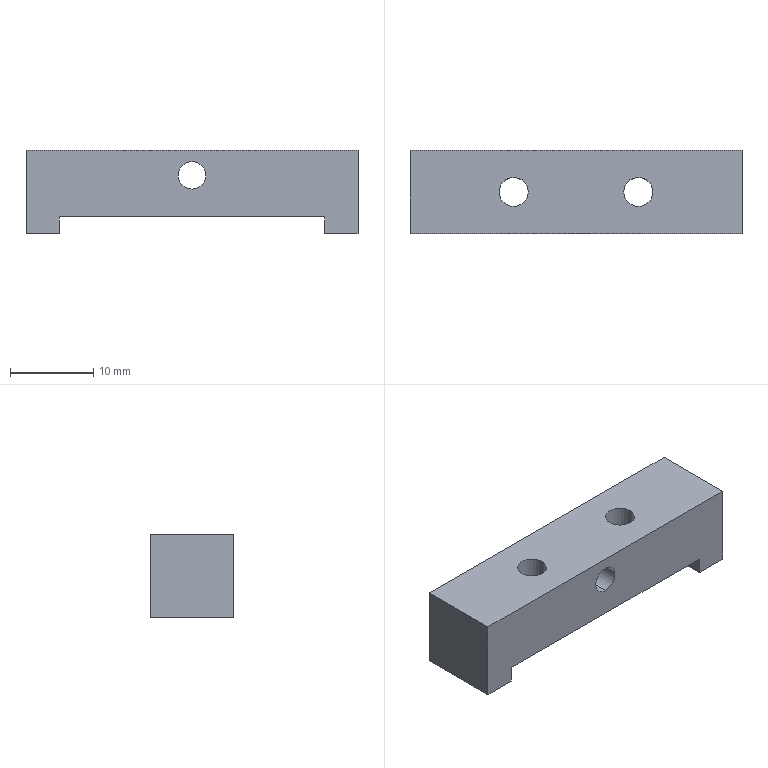Part | STEP file | 11-FG-E04311 | 1 solid | 16 faces | box 40 x 10 x 10 mm | volume 3121 mm3 | plane 10 | cylinder 6 | commonest cylinder face diameters 3.5 x4 3.3 x2
STEP:
#1=CARTESIAN_POINT('',(0.,-5.,5.35));
#2=VERTEX_POINT('',#1);
#3=CARTESIAN_POINT('',(0.,-5.,8.65));
#4=VERTEX_POINT('',#3);
#5=CARTESIAN_POINT('',(0.,-5.,7.));
#6=DIRECTION('',(0.,1.,0.));
#7=DIRECTION('',(0.,0.,1.));
#8=AXIS2_PLACEMENT_3D('',#5,#6,#7);
#9=CIRCLE('',#8,1.65);
#10=EDGE_CURVE('',#2,#4,#9,.T.);
#11=ORIENTED_EDGE('',*,*,#10,.F.);
#12=CARTESIAN_POINT('',(0.,5.,5.35));
#13=VERTEX_POINT('',#12);
#14=CARTESIAN_POINT('',(0.,5.,5.35));
#15=DIRECTION('',(0.,1.,0.));
#16=VECTOR('',#15,1000.);
#17=LINE('',#14,#16);
#18=EDGE_CURVE('',#2,#13,#17,.T.);
#19=ORIENTED_EDGE('',*,*,#18,.T.);
#20=CARTESIAN_POINT('',(0.,5.,8.65));
#21=VERTEX_POINT('',#20);
#22=CARTESIAN_POINT('',(0.,5.,7.));
#23=DIRECTION('',(0.,1.,0.));
#24=DIRECTION('',(0.,0.,1.));
#25=AXIS2_PLACEMENT_3D('',#22,#23,#24);
#26=CIRCLE('',#25,1.65);
#27=EDGE_CURVE('',#13,#21,#26,.T.);
#28=ORIENTED_EDGE('',*,*,#27,.T.);
#29=CARTESIAN_POINT('',(0.,5.,8.65));
#30=DIRECTION('',(0.,1.,0.));
#31=VECTOR('',#30,1000.);
#32=LINE('',#29,#31);
#33=EDGE_CURVE('',#4,#21,#32,.T.);
#34=ORIENTED_EDGE('',*,*,#33,.F.);
#35=EDGE_LOOP('',(#11,#19,#28,#34));
#36=FACE_OUTER_BOUND('',#35,.T.);
#37=CARTESIAN_POINT('',(0.,5.,7.));
#38=DIRECTION('',(0.,1.,0.));
#39=DIRECTION('',(0.,0.,1.));
#40=AXIS2_PLACEMENT_3D('',#37,#38,#39);
#41=CYLINDRICAL_SURFACE('',#40,1.65);
#42=ADVANCED_FACE('',(#36),#41,.F.);
#43=CARTESIAN_POINT('',(5.75,0.,2.));
#44=VERTEX_POINT('',#43);
#45=CARTESIAN_POINT('',(9.25,0.,2.));
#46=VERTEX_POINT('',#45);
#47=CARTESIAN_POINT('',(7.5,0.,2.));
#48=DIRECTION('',(0.,0.,1.));
#49=DIRECTION('',(1.,0.,0.));
#50=AXIS2_PLACEMENT_3D('',#47,#48,#49);
#51=CIRCLE('',#50,1.75);
#52=EDGE_CURVE('',#44,#46,#51,.T.);
#53=ORIENTED_EDGE('',*,*,#52,.F.);
#54=CARTESIAN_POINT('',(5.75,0.,10.));
#55=VERTEX_POINT('',#54);
#56=CARTESIAN_POINT('',(5.75,0.,2.));
#57=DIRECTION('',(0.,0.,1.));
#58=VECTOR('',#57,1000.);
#59=LINE('',#56,#58);
#60=EDGE_CURVE('',#44,#55,#59,.T.);
#61=ORIENTED_EDGE('',*,*,#60,.T.);
#62=CARTESIAN_POINT('',(9.25,0.,10.));
#63=VERTEX_POINT('',#62);
#64=CARTESIAN_POINT('',(7.5,0.,10.));
#65=DIRECTION('',(0.,0.,1.));
#66=DIRECTION('',(1.,0.,0.));
#67=AXIS2_PLACEMENT_3D('',#64,#65,#66);
#68=CIRCLE('',#67,1.75);
#69=EDGE_CURVE('',#55,#63,#68,.T.);
#70=ORIENTED_EDGE('',*,*,#69,.T.);
#71=CARTESIAN_POINT('',(9.25,0.,2.));
#72=DIRECTION('',(0.,0.,1.));
#73=VECTOR('',#72,1000.);
#74=LINE('',#71,#73);
#75=EDGE_CURVE('',#46,#63,#74,.T.);
#76=ORIENTED_EDGE('',*,*,#75,.F.);
#77=EDGE_LOOP('',(#53,#61,#70,#76));
#78=FACE_OUTER_BOUND('',#77,.T.);
#79=CARTESIAN_POINT('',(7.5,0.,2.));
#80=DIRECTION('',(0.,0.,1.));
#81=DIRECTION('',(1.,0.,0.));
#82=AXIS2_PLACEMENT_3D('',#79,#80,#81);
#83=CYLINDRICAL_SURFACE('',#82,1.75);
#84=ADVANCED_FACE('',(#78),#83,.F.);
#85=CARTESIAN_POINT('',(-9.25,0.,2.));
#86=VERTEX_POINT('',#85);
#87=CARTESIAN_POINT('',(-5.75,0.,2.));
#88=VERTEX_POINT('',#87);
#89=CARTESIAN_POINT('',(-7.5,0.,2.));
#90=DIRECTION('',(0.,0.,1.));
#91=DIRECTION('',(1.,0.,0.));
#92=AXIS2_PLACEMENT_3D('',#89,#90,#91);
#93=CIRCLE('',#92,1.75);
#94=EDGE_CURVE('',#86,#88,#93,.T.);
#95=ORIENTED_EDGE('',*,*,#94,.F.);
#96=CARTESIAN_POINT('',(-9.25,0.,10.));
#97=VERTEX_POINT('',#96);
#98=CARTESIAN_POINT('',(-9.25,0.,2.));
#99=DIRECTION('',(0.,0.,1.));
#100=VECTOR('',#99,1000.);
#101=LINE('',#98,#100);
#102=EDGE_CURVE('',#86,#97,#101,.T.);
#103=ORIENTED_EDGE('',*,*,#102,.T.);
#104=CARTESIAN_POINT('',(-5.75,0.,10.));
#105=VERTEX_POINT('',#104);
#106=CARTESIAN_POINT('',(-7.5,0.,10.));
#107=DIRECTION('',(0.,0.,1.));
#108=DIRECTION('',(1.,0.,0.));
#109=AXIS2_PLACEMENT_3D('',#106,#107,#108);
#110=CIRCLE('',#109,1.75);
#111=EDGE_CURVE('',#97,#105,#110,.T.);
#112=ORIENTED_EDGE('',*,*,#111,.T.);
#113=CARTESIAN_POINT('',(-5.75,0.,2.));
#114=DIRECTION('',(0.,0.,1.));
#115=VECTOR('',#114,1000.);
#116=LINE('',#113,#115);
#117=EDGE_CURVE('',#88,#105,#116,.T.);
#118=ORIENTED_EDGE('',*,*,#117,.F.);
#119=EDGE_LOOP('',(#95,#103,#112,#118));
#120=FACE_OUTER_BOUND('',#119,.T.);
#121=CARTESIAN_POINT('',(-7.5,0.,2.));
#122=DIRECTION('',(0.,0.,1.));
#123=DIRECTION('',(1.,0.,0.));
#124=AXIS2_PLACEMENT_3D('',#121,#122,#123);
#125=CYLINDRICAL_SURFACE('',#124,1.75);
#126=ADVANCED_FACE('',(#120),#125,.F.);
#127=CARTESIAN_POINT('',(-16.,5.,0.));
#128=VERTEX_POINT('',#127);
#129=CARTESIAN_POINT('',(-20.,5.,0.));
#130=VERTEX_POINT('',#129);
#131=CARTESIAN_POINT('',(-20.,5.,0.));
#132=DIRECTION('',(-1.,0.,0.));
#133=VECTOR('',#132,1000.);
#134=LINE('',#131,#133);
#135=EDGE_CURVE('',#128,#130,#134,.T.);
#136=ORIENTED_EDGE('',*,*,#135,.F.);
#137=CARTESIAN_POINT('',(-16.,-5.,0.));
#138=VERTEX_POINT('',#137);
#139=CARTESIAN_POINT('',(-16.,0.,0.));
#140=DIRECTION('',(0.,-1.,0.));
#141=VECTOR('',#140,1000.);
#142=LINE('',#139,#141);
#143=EDGE_CURVE('',#128,#138,#142,.T.);
#144=ORIENTED_EDGE('',*,*,#143,.T.);
#145=CARTESIAN_POINT('',(-20.,-5.,0.));
#146=VERTEX_POINT('',#145);
#147=CARTESIAN_POINT('',(-20.,-5.,0.));
#148=DIRECTION('',(1.,0.,0.));
#149=VECTOR('',#148,1000.);
#150=LINE('',#147,#149);
#151=EDGE_CURVE('',#146,#138,#150,.T.);
#152=ORIENTED_EDGE('',*,*,#151,.F.);
#153=CARTESIAN_POINT('',(-20.,5.,0.));
#154=DIRECTION('',(0.,-1.,0.));
#155=VECTOR('',#154,1000.);
#156=LINE('',#153,#155);
#157=EDGE_CURVE('',#130,#146,#156,.T.);
#158=ORIENTED_EDGE('',*,*,#157,.F.);
#159=EDGE_LOOP('',(#136,#144,#152,#158));
#160=FACE_OUTER_BOUND('',#159,.T.);
#161=CARTESIAN_POINT('',(0.,0.,0.));
#162=DIRECTION('',(0.,0.,1.));
#163=DIRECTION('',(1.,0.,0.));
#164=AXIS2_PLACEMENT_3D('',#161,#162,#163);
#165=PLANE('',#164);
#166=ADVANCED_FACE('',(#160),#165,.F.);
#167=CARTESIAN_POINT('',(20.,-5.,0.));
#168=VERTEX_POINT('',#167);
#169=CARTESIAN_POINT('',(20.,5.,0.));
#170=VERTEX_POINT('',#169);
#171=CARTESIAN_POINT('',(20.,5.,0.));
#172=DIRECTION('',(0.,1.,0.));
#173=VECTOR('',#172,1000.);
#174=LINE('',#171,#173);
#175=EDGE_CURVE('',#168,#170,#174,.T.);
#176=ORIENTED_EDGE('',*,*,#175,.T.);
#177=CARTESIAN_POINT('',(20.,5.,10.));
#178=VERTEX_POINT('',#177);
#179=CARTESIAN_POINT('',(20.,5.,10.));
#180=DIRECTION('',(0.,0.,-1.));
#181=VECTOR('',#180,1000.);
#182=LINE('',#179,#181);
#183=EDGE_CURVE('',#178,#170,#182,.T.);
#184=ORIENTED_EDGE('',*,*,#183,.F.);
#185=CARTESIAN_POINT('',(20.,-5.,10.));
#186=VERTEX_POINT('',#185);
#187=CARTESIAN_POINT('',(20.,5.,10.));
#188=DIRECTION('',(0.,1.,0.));
#189=VECTOR('',#188,1000.);
#190=LINE('',#187,#189);
#191=EDGE_CURVE('',#186,#178,#190,.T.);
#192=ORIENTED_EDGE('',*,*,#191,.F.);
#193=CARTESIAN_POINT('',(20.,-5.,10.));
#194=DIRECTION('',(0.,0.,-1.));
#195=VECTOR('',#194,1000.);
#196=LINE('',#193,#195);
#197=EDGE_CURVE('',#186,#168,#196,.T.);
#198=ORIENTED_EDGE('',*,*,#197,.T.);
#199=EDGE_LOOP('',(#176,#184,#192,#198));
#200=FACE_OUTER_BOUND('',#199,.T.);
#201=CARTESIAN_POINT('',(20.,5.,10.));
#202=DIRECTION('',(-1.,0.,0.));
#203=DIRECTION('',(0.,0.,1.));
#204=AXIS2_PLACEMENT_3D('',#201,#202,#203);
#205=PLANE('',#204);
#206=ADVANCED_FACE('',(#200),#205,.F.);
#207=CARTESIAN_POINT('',(0.,5.,7.));
#208=DIRECTION('',(0.,1.,0.));
#209=DIRECTION('',(0.,0.,1.));
#210=AXIS2_PLACEMENT_3D('',#207,#208,#209);
#211=CIRCLE('',#210,1.65);
#212=EDGE_CURVE('',#21,#13,#211,.T.);
#213=ORIENTED_EDGE('',*,*,#212,.F.);
#214=ORIENTED_EDGE('',*,*,#27,.F.);
#215=EDGE_LOOP('',(#213,#214));
#216=FACE_BOUND('',#215,.T.);
#217=CARTESIAN_POINT('',(-16.,5.,2.));
#218=VERTEX_POINT('',#217);
#219=CARTESIAN_POINT('',(16.,5.,2.));
#220=VERTEX_POINT('',#219);
#221=CARTESIAN_POINT('',(-16.,5.,2.));
#222=DIRECTION('',(1.,0.,0.));
#223=VECTOR('',#222,1000.);
#224=LINE('',#221,#223);
#225=EDGE_CURVE('',#218,#220,#224,.T.);
#226=ORIENTED_EDGE('',*,*,#225,.F.);
#227=CARTESIAN_POINT('',(-16.,5.,0.));
#228=DIRECTION('',(0.,0.,1.));
#229=VECTOR('',#228,1000.);
#230=LINE('',#227,#229);
#231=EDGE_CURVE('',#128,#218,#230,.T.);
#232=ORIENTED_EDGE('',*,*,#231,.F.);
#233=ORIENTED_EDGE('',*,*,#135,.T.);
#234=CARTESIAN_POINT('',(-20.,5.,10.));
#235=VERTEX_POINT('',#234);
#236=CARTESIAN_POINT('',(-20.,5.,10.));
#237=DIRECTION('',(0.,0.,-1.));
#238=VECTOR('',#237,1000.);
#239=LINE('',#236,#238);
#240=EDGE_CURVE('',#235,#130,#239,.T.);
#241=ORIENTED_EDGE('',*,*,#240,.F.);
#242=CARTESIAN_POINT('',(-20.,5.,10.));
#243=DIRECTION('',(-1.,0.,0.));
#244=VECTOR('',#243,1000.);
#245=LINE('',#242,#244);
#246=EDGE_CURVE('',#178,#235,#245,.T.);
#247=ORIENTED_EDGE('',*,*,#246,.F.);
#248=ORIENTED_EDGE('',*,*,#183,.T.);
#249=CARTESIAN_POINT('',(16.,5.,0.));
#250=VERTEX_POINT('',#249);
#251=CARTESIAN_POINT('',(-20.,5.,0.));
#252=DIRECTION('',(-1.,0.,0.));
#253=VECTOR('',#252,1000.);
#254=LINE('',#251,#253);
#255=EDGE_CURVE('',#170,#250,#254,.T.);
#256=ORIENTED_EDGE('',*,*,#255,.T.);
#257=CARTESIAN_POINT('',(16.,5.,0.));
#258=DIRECTION('',(0.,0.,-1.));
#259=VECTOR('',#258,1000.);
#260=LINE('',#257,#259);
#261=EDGE_CURVE('',#220,#250,#260,.T.);
#262=ORIENTED_EDGE('',*,*,#261,.F.);
#263=EDGE_LOOP('',(#226,#232,#233,#241,#247,#248,#256,#262));
#264=FACE_OUTER_BOUND('',#263,.T.);
#265=CARTESIAN_POINT('',(-20.,5.,10.));
#266=DIRECTION('',(0.,-1.,0.));
#267=DIRECTION('',(0.,0.,-1.));
#268=AXIS2_PLACEMENT_3D('',#265,#266,#267);
#269=PLANE('',#268);
#270=ADVANCED_FACE('',(#216,#264),#269,.F.);
#271=ORIENTED_EDGE('',*,*,#157,.T.);
#272=CARTESIAN_POINT('',(-20.,-5.,10.));
#273=VERTEX_POINT('',#272);
#274=CARTESIAN_POINT('',(-20.,-5.,10.));
#275=DIRECTION('',(0.,0.,-1.));
#276=VECTOR('',#275,1000.);
#277=LINE('',#274,#276);
#278=EDGE_CURVE('',#273,#146,#277,.T.);
#279=ORIENTED_EDGE('',*,*,#278,.F.);
#280=CARTESIAN_POINT('',(-20.,5.,10.));
#281=DIRECTION('',(0.,-1.,0.));
#282=VECTOR('',#281,1000.);
#283=LINE('',#280,#282);
#284=EDGE_CURVE('',#235,#273,#283,.T.);
#285=ORIENTED_EDGE('',*,*,#284,.F.);
#286=ORIENTED_EDGE('',*,*,#240,.T.);
#287=EDGE_LOOP('',(#271,#279,#285,#286));
#288=FACE_OUTER_BOUND('',#287,.T.);
#289=CARTESIAN_POINT('',(-20.,5.,10.));
#290=DIRECTION('',(1.,0.,0.));
#291=DIRECTION('',(0.,0.,-1.));
#292=AXIS2_PLACEMENT_3D('',#289,#290,#291);
#293=PLANE('',#292);
#294=ADVANCED_FACE('',(#288),#293,.F.);
#295=CARTESIAN_POINT('',(0.,-5.,7.));
#296=DIRECTION('',(0.,1.,0.));
#297=DIRECTION('',(0.,0.,1.));
#298=AXIS2_PLACEMENT_3D('',#295,#296,#297);
#299=CIRCLE('',#298,1.65);
#300=EDGE_CURVE('',#4,#2,#299,.T.);
#301=ORIENTED_EDGE('',*,*,#300,.T.);
#302=ORIENTED_EDGE('',*,*,#10,.T.);
#303=EDGE_LOOP('',(#301,#302));
#304=FACE_BOUND('',#303,.T.);
#305=ORIENTED_EDGE('',*,*,#151,.T.);
#306=CARTESIAN_POINT('',(-16.,-5.,2.));
#307=VERTEX_POINT('',#306);
#308=CARTESIAN_POINT('',(-16.,-5.,10.));
#309=DIRECTION('',(0.,0.,1.));
#310=VECTOR('',#309,1000.);
#311=LINE('',#308,#310);
#312=EDGE_CURVE('',#138,#307,#311,.T.);
#313=ORIENTED_EDGE('',*,*,#312,.T.);
#314=CARTESIAN_POINT('',(16.,-5.,2.));
#315=VERTEX_POINT('',#314);
#316=CARTESIAN_POINT('',(-20.,-5.,2.));
#317=DIRECTION('',(1.,0.,0.));
#318=VECTOR('',#317,1000.);
#319=LINE('',#316,#318);
#320=EDGE_CURVE('',#307,#315,#319,.T.);
#321=ORIENTED_EDGE('',*,*,#320,.T.);
#322=CARTESIAN_POINT('',(16.,-5.,0.));
#323=VERTEX_POINT('',#322);
#324=CARTESIAN_POINT('',(16.,-5.,10.));
#325=DIRECTION('',(0.,0.,-1.));
#326=VECTOR('',#325,1000.);
#327=LINE('',#324,#326);
#328=EDGE_CURVE('',#315,#323,#327,.T.);
#329=ORIENTED_EDGE('',*,*,#328,.T.);
#330=CARTESIAN_POINT('',(-20.,-5.,0.));
#331=DIRECTION('',(1.,0.,0.));
#332=VECTOR('',#331,1000.);
#333=LINE('',#330,#332);
#334=EDGE_CURVE('',#323,#168,#333,.T.);
#335=ORIENTED_EDGE('',*,*,#334,.T.);
#336=ORIENTED_EDGE('',*,*,#197,.F.);
#337=CARTESIAN_POINT('',(-20.,-5.,10.));
#338=DIRECTION('',(1.,0.,0.));
#339=VECTOR('',#338,1000.);
#340=LINE('',#337,#339);
#341=EDGE_CURVE('',#273,#186,#340,.T.);
#342=ORIENTED_EDGE('',*,*,#341,.F.);
#343=ORIENTED_EDGE('',*,*,#278,.T.);
#344=EDGE_LOOP('',(#305,#313,#321,#329,#335,#336,#342,#343));
#345=FACE_OUTER_BOUND('',#344,.T.);
#346=CARTESIAN_POINT('',(-20.,-5.,10.));
#347=DIRECTION('',(0.,1.,0.));
#348=DIRECTION('',(0.,0.,1.));
#349=AXIS2_PLACEMENT_3D('',#346,#347,#348);
#350=PLANE('',#349);
#351=ADVANCED_FACE('',(#304,#345),#350,.F.);
#352=CARTESIAN_POINT('',(7.5,0.,10.));
#353=DIRECTION('',(0.,0.,1.));
#354=DIRECTION('',(1.,0.,0.));
#355=AXIS2_PLACEMENT_3D('',#352,#353,#354);
#356=CIRCLE('',#355,1.75);
#357=EDGE_CURVE('',#63,#55,#356,.T.);
#358=ORIENTED_EDGE('',*,*,#357,.F.);
#359=ORIENTED_EDGE('',*,*,#69,.F.);
#360=EDGE_LOOP('',(#358,#359));
#361=FACE_BOUND('',#360,.T.);
#362=CARTESIAN_POINT('',(-7.5,0.,10.));
#363=DIRECTION('',(0.,0.,1.));
#364=DIRECTION('',(1.,0.,0.));
#365=AXIS2_PLACEMENT_3D('',#362,#363,#364);
#366=CIRCLE('',#365,1.75);
#367=EDGE_CURVE('',#105,#97,#366,.T.);
#368=ORIENTED_EDGE('',*,*,#367,.F.);
#369=ORIENTED_EDGE('',*,*,#111,.F.);
#370=EDGE_LOOP('',(#368,#369));
#371=FACE_BOUND('',#370,.T.);
#372=ORIENTED_EDGE('',*,*,#191,.T.);
#373=ORIENTED_EDGE('',*,*,#246,.T.);
#374=ORIENTED_EDGE('',*,*,#284,.T.);
#375=ORIENTED_EDGE('',*,*,#341,.T.);
#376=EDGE_LOOP('',(#372,#373,#374,#375));
#377=FACE_OUTER_BOUND('',#376,.T.);
#378=CARTESIAN_POINT('',(0.,0.,10.));
#379=DIRECTION('',(0.,0.,1.));
#380=DIRECTION('',(1.,0.,0.));
#381=AXIS2_PLACEMENT_3D('',#378,#379,#380);
#382=PLANE('',#381);
#383=ADVANCED_FACE('',(#361,#371,#377),#382,.T.);
#384=ORIENTED_EDGE('',*,*,#334,.F.);
#385=CARTESIAN_POINT('',(16.,0.,0.));
#386=DIRECTION('',(0.,1.,0.));
#387=VECTOR('',#386,1000.);
#388=LINE('',#385,#387);
#389=EDGE_CURVE('',#323,#250,#388,.T.);
#390=ORIENTED_EDGE('',*,*,#389,.T.);
#391=ORIENTED_EDGE('',*,*,#255,.F.);
#392=ORIENTED_EDGE('',*,*,#175,.F.);
#393=EDGE_LOOP('',(#384,#390,#391,#392));
#394=FACE_OUTER_BOUND('',#393,.T.);
#395=CARTESIAN_POINT('',(0.,0.,0.));
#396=DIRECTION('',(0.,0.,1.));
#397=DIRECTION('',(1.,0.,0.));
#398=AXIS2_PLACEMENT_3D('',#395,#396,#397);
#399=PLANE('',#398);
#400=ADVANCED_FACE('',(#394),#399,.F.);
#401=CARTESIAN_POINT('',(7.5,0.,2.));
#402=DIRECTION('',(0.,0.,1.));
#403=DIRECTION('',(1.,0.,0.));
#404=AXIS2_PLACEMENT_3D('',#401,#402,#403);
#405=CIRCLE('',#404,1.75);
#406=EDGE_CURVE('',#46,#44,#405,.T.);
#407=ORIENTED_EDGE('',*,*,#406,.T.);
#408=ORIENTED_EDGE('',*,*,#52,.T.);
#409=EDGE_LOOP('',(#407,#408));
#410=FACE_BOUND('',#409,.T.);
#411=CARTESIAN_POINT('',(-7.5,0.,2.));
#412=DIRECTION('',(0.,0.,1.));
#413=DIRECTION('',(1.,0.,0.));
#414=AXIS2_PLACEMENT_3D('',#411,#412,#413);
#415=CIRCLE('',#414,1.75);
#416=EDGE_CURVE('',#88,#86,#415,.T.);
#417=ORIENTED_EDGE('',*,*,#416,.T.);
#418=ORIENTED_EDGE('',*,*,#94,.T.);
#419=EDGE_LOOP('',(#417,#418));
#420=FACE_BOUND('',#419,.T.);
#421=CARTESIAN_POINT('',(-16.,-15.,2.));
#422=DIRECTION('',(0.,1.,0.));
#423=VECTOR('',#422,1000.);
#424=LINE('',#421,#423);
#425=EDGE_CURVE('',#307,#218,#424,.T.);
#426=ORIENTED_EDGE('',*,*,#425,.T.);
#427=ORIENTED_EDGE('',*,*,#225,.T.);
#428=CARTESIAN_POINT('',(16.,-15.,2.));
#429=DIRECTION('',(0.,1.,0.));
#430=VECTOR('',#429,1000.);
#431=LINE('',#428,#430);
#432=EDGE_CURVE('',#315,#220,#431,.T.);
#433=ORIENTED_EDGE('',*,*,#432,.F.);
#434=ORIENTED_EDGE('',*,*,#320,.F.);
#435=EDGE_LOOP('',(#426,#427,#433,#434));
#436=FACE_OUTER_BOUND('',#435,.T.);
#437=CARTESIAN_POINT('',(-16.,-15.,2.));
#438=DIRECTION('',(0.,0.,1.));
#439=DIRECTION('',(1.,0.,0.));
#440=AXIS2_PLACEMENT_3D('',#437,#438,#439);
#441=PLANE('',#440);
#442=ADVANCED_FACE('',(#410,#420,#436),#441,.F.);
#443=ORIENTED_EDGE('',*,*,#143,.F.);
#444=ORIENTED_EDGE('',*,*,#231,.T.);
#445=ORIENTED_EDGE('',*,*,#425,.F.);
#446=ORIENTED_EDGE('',*,*,#312,.F.);
#447=EDGE_LOOP('',(#443,#444,#445,#446));
#448=FACE_OUTER_BOUND('',#447,.T.);
#449=CARTESIAN_POINT('',(-16.,-15.,0.));
#450=DIRECTION('',(-1.,0.,0.));
#451=DIRECTION('',(0.,0.,1.));
#452=AXIS2_PLACEMENT_3D('',#449,#450,#451);
#453=PLANE('',#452);
#454=ADVANCED_FACE('',(#448),#453,.F.);
#455=ORIENTED_EDGE('',*,*,#432,.T.);
#456=ORIENTED_EDGE('',*,*,#261,.T.);
#457=ORIENTED_EDGE('',*,*,#389,.F.);
#458=ORIENTED_EDGE('',*,*,#328,.F.);
#459=EDGE_LOOP('',(#455,#456,#457,#458));
#460=FACE_OUTER_BOUND('',#459,.T.);
#461=CARTESIAN_POINT('',(16.,-15.,0.));
#462=DIRECTION('',(1.,0.,0.));
#463=DIRECTION('',(0.,0.,-1.));
#464=AXIS2_PLACEMENT_3D('',#461,#462,#463);
#465=PLANE('',#464);
#466=ADVANCED_FACE('',(#460),#465,.F.);
#467=ORIENTED_EDGE('',*,*,#102,.F.);
#468=ORIENTED_EDGE('',*,*,#416,.F.);
#469=ORIENTED_EDGE('',*,*,#117,.T.);
#470=ORIENTED_EDGE('',*,*,#367,.T.);
#471=EDGE_LOOP('',(#467,#468,#469,#470));
#472=FACE_OUTER_BOUND('',#471,.T.);
#473=CARTESIAN_POINT('',(-7.5,0.,2.));
#474=DIRECTION('',(0.,0.,1.));
#475=DIRECTION('',(1.,0.,0.));
#476=AXIS2_PLACEMENT_3D('',#473,#474,#475);
#477=CYLINDRICAL_SURFACE('',#476,1.75);
#478=ADVANCED_FACE('',(#472),#477,.F.);
#479=ORIENTED_EDGE('',*,*,#60,.F.);
#480=ORIENTED_EDGE('',*,*,#406,.F.);
#481=ORIENTED_EDGE('',*,*,#75,.T.);
#482=ORIENTED_EDGE('',*,*,#357,.T.);
#483=EDGE_LOOP('',(#479,#480,#481,#482));
#484=FACE_OUTER_BOUND('',#483,.T.);
#485=CARTESIAN_POINT('',(7.5,0.,2.));
#486=DIRECTION('',(0.,0.,1.));
#487=DIRECTION('',(1.,0.,0.));
#488=AXIS2_PLACEMENT_3D('',#485,#486,#487);
#489=CYLINDRICAL_SURFACE('',#488,1.75);
#490=ADVANCED_FACE('',(#484),#489,.F.);
#491=ORIENTED_EDGE('',*,*,#18,.F.);
#492=ORIENTED_EDGE('',*,*,#300,.F.);
#493=ORIENTED_EDGE('',*,*,#33,.T.);
#494=ORIENTED_EDGE('',*,*,#212,.T.);
#495=EDGE_LOOP('',(#491,#492,#493,#494));
#496=FACE_OUTER_BOUND('',#495,.T.);
#497=CARTESIAN_POINT('',(0.,5.,7.));
#498=DIRECTION('',(0.,1.,0.));
#499=DIRECTION('',(0.,0.,1.));
#500=AXIS2_PLACEMENT_3D('',#497,#498,#499);
#501=CYLINDRICAL_SURFACE('',#500,1.65);
#502=ADVANCED_FACE('',(#496),#501,.F.);
#503=CLOSED_SHELL('',(#42,#84,#126,#166,#206,#270,#294,#351,#383,#400,#442,#454,#466,#478,#490,#502));
#504=MANIFOLD_SOLID_BREP('',#503);
#505=CARTESIAN_POINT('',(0.,0.,0.));
#506=DIRECTION('',(0.,0.,1.));
#507=DIRECTION('',(1.,0.,0.));
#508=AXIS2_PLACEMENT_3D('',#505,#506,#507);
#509=(LENGTH_UNIT()NAMED_UNIT(*)SI_UNIT(.MILLI.,.METRE.));
#510=UNCERTAINTY_MEASURE_WITH_UNIT(LENGTH_MEASURE(0.00001),#509,'','');
#511=(NAMED_UNIT(*)PLANE_ANGLE_UNIT()SI_UNIT($,.RADIAN.));
#512=(NAMED_UNIT(*)SI_UNIT($,.STERADIAN.)SOLID_ANGLE_UNIT());
#513=(GEOMETRIC_REPRESENTATION_CONTEXT(3)GLOBAL_UNCERTAINTY_ASSIGNED_CONTEXT((#510))GLOBAL_UNIT_ASSIGNED_CONTEXT((#509,#511,#512))REPRESENTATION_CONTEXT('',''));
#514=ADVANCED_BREP_SHAPE_REPRESENTATION('',(#504,#508),#513);